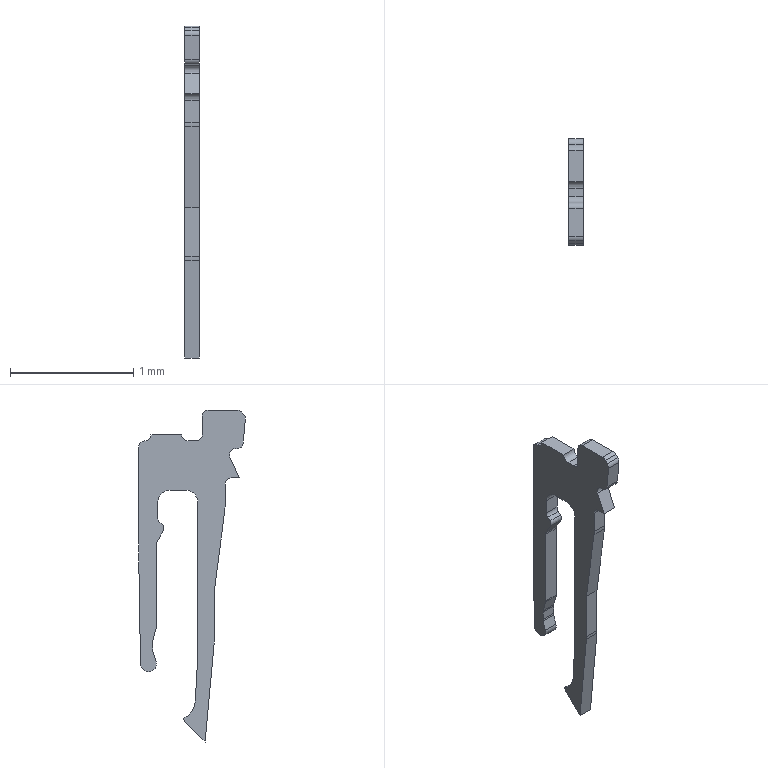Part | Creo | 1 solid | 55 faces | box 0.12 x 0.865 x 2.691 mm | volume 0.1098 mm3 | plane 29 | cylinder 26 | commonest cylinder face diameters 0.1 x15 0.6 x3 0.08 x2 0.12 x2 0.2 x2 0.354 x1